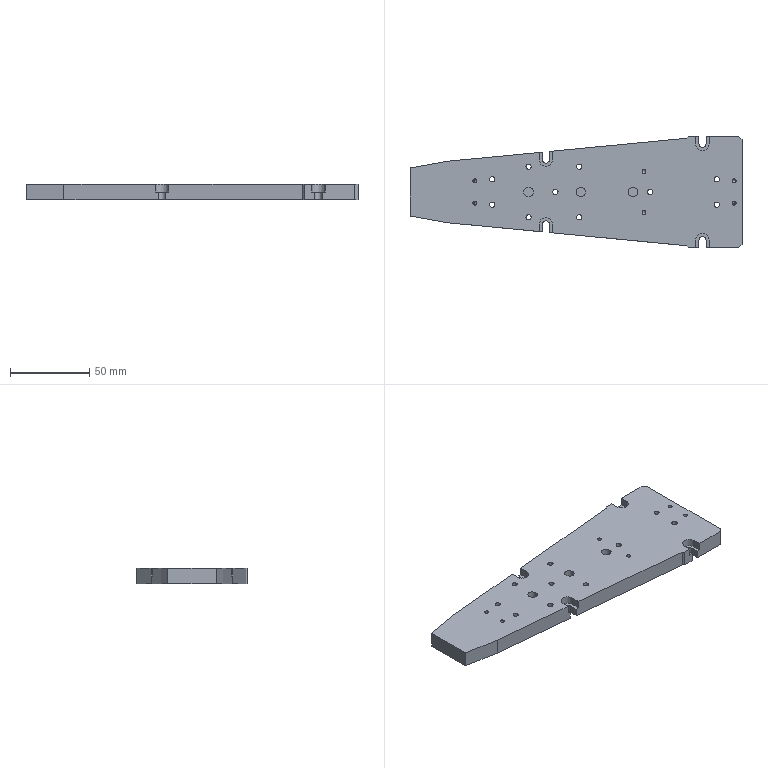Part | SolidWorks | features HoleWzd 5, ICE 5, Chamfer 2, Cut 1, Extrusion 1 | 1 solid | 116 faces | box 210 x 70 x 10 mm | volume 108255 mm3 | cylinder 54 | plane 50 | cone 12 | commonest cylinder face diameters 3.3 x20 2.5 x12 5 x6 6 x6 4.5 x4 8.5 x4